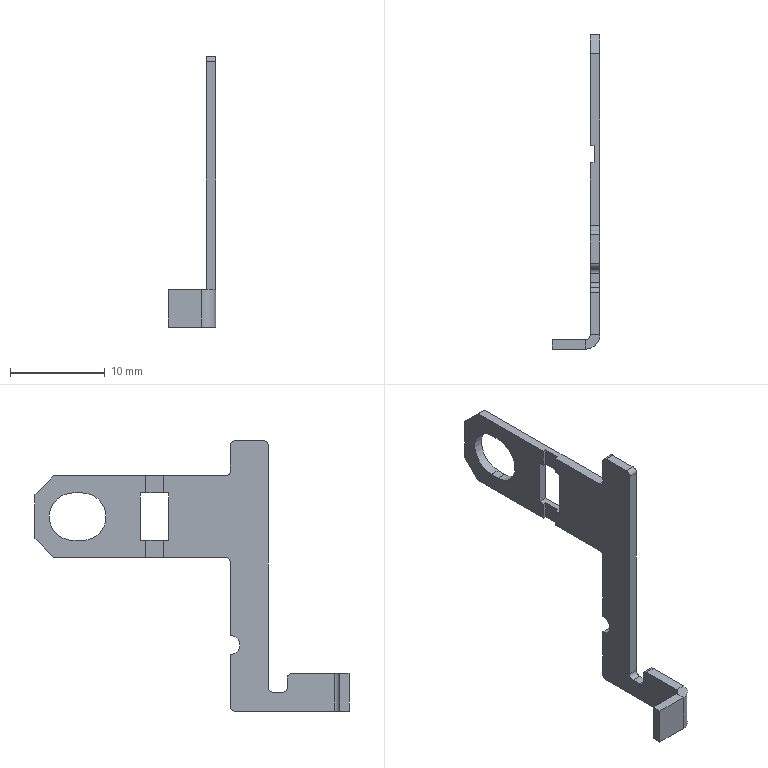Part | SolidWorks | features ICE 7, Chamfer 1, EdgeFlange 1, Fillet 1, FlatPattern 1, SMBaseFlange 1, SheetMetal 1 | 1 solid | 49 faces | box 5 x 33.1 x 28.5 mm | volume 287.645 mm3 | plane 36 | cylinder 13 | commonest cylinder face diameters 1 x9 5 x2 2 x1 3 x1
STEP:
#1=CARTESIAN_POINT('',(-4.,12.5,5.98));
#2=VERTEX_POINT('',#1);
#3=CARTESIAN_POINT('',(-5.,12.5,5.98));
#4=VERTEX_POINT('',#3);
#5=CARTESIAN_POINT('',(0.,12.5,5.98));
#6=DIRECTION('',(-1.,0.,0.));
#7=VECTOR('',#6,1000.);
#8=LINE('',#5,#7);
#9=EDGE_CURVE('',#2,#4,#8,.T.);
#10=ORIENTED_EDGE('',*,*,#9,.F.);
#11=CARTESIAN_POINT('',(-4.,12.5,0.5));
#12=VERTEX_POINT('',#11);
#13=CARTESIAN_POINT('',(-4.,12.5,4.));
#14=DIRECTION('',(0.,0.,-1.));
#15=VECTOR('',#14,1000.);
#16=LINE('',#13,#15);
#17=EDGE_CURVE('',#2,#12,#16,.T.);
#18=ORIENTED_EDGE('',*,*,#17,.T.);
#19=CARTESIAN_POINT('',(-5.,12.5,0.5));
#20=VERTEX_POINT('',#19);
#21=CARTESIAN_POINT('',(-5.,12.5,0.5));
#22=DIRECTION('',(-1.,0.,0.));
#23=VECTOR('',#22,1000.);
#24=LINE('',#21,#23);
#25=EDGE_CURVE('',#12,#20,#24,.T.);
#26=ORIENTED_EDGE('',*,*,#25,.T.);
#27=CARTESIAN_POINT('',(-5.,12.5,4.));
#28=DIRECTION('',(0.,0.,-1.));
#29=VECTOR('',#28,1000.);
#30=LINE('',#27,#29);
#31=EDGE_CURVE('',#4,#20,#30,.T.);
#32=ORIENTED_EDGE('',*,*,#31,.F.);
#33=EDGE_LOOP('',(#10,#18,#26,#32));
#34=FACE_OUTER_BOUND('',#33,.T.);
#35=CARTESIAN_POINT('',(-5.,12.5,4.));
#36=DIRECTION('',(0.,1.,0.));
#37=DIRECTION('',(0.,0.,1.));
#38=AXIS2_PLACEMENT_3D('',#35,#36,#37);
#39=PLANE('',#38);
#40=ADVANCED_FACE('',(#34),#39,.T.);
#41=CARTESIAN_POINT('',(-4.6,21.4,16.2));
#42=VERTEX_POINT('',#41);
#43=CARTESIAN_POINT('',(-4.6,21.4,18.));
#44=VERTEX_POINT('',#43);
#45=CARTESIAN_POINT('',(-4.6,21.4,0.));
#46=DIRECTION('',(0.,0.,1.));
#47=VECTOR('',#46,1000.);
#48=LINE('',#45,#47);
#49=EDGE_CURVE('',#42,#44,#48,.T.);
#50=ORIENTED_EDGE('',*,*,#49,.T.);
#51=CARTESIAN_POINT('',(-5.,21.4,18.));
#52=VERTEX_POINT('',#51);
#53=CARTESIAN_POINT('',(-5.,21.4,18.));
#54=DIRECTION('',(-1.,0.,0.));
#55=VECTOR('',#54,1000.);
#56=LINE('',#53,#55);
#57=EDGE_CURVE('',#44,#52,#56,.T.);
#58=ORIENTED_EDGE('',*,*,#57,.T.);
#59=CARTESIAN_POINT('',(-5.,21.4,16.2));
#60=VERTEX_POINT('',#59);
#61=CARTESIAN_POINT('',(-5.,21.4,0.));
#62=DIRECTION('',(0.,0.,1.));
#63=VECTOR('',#62,1000.);
#64=LINE('',#61,#63);
#65=EDGE_CURVE('',#60,#52,#64,.T.);
#66=ORIENTED_EDGE('',*,*,#65,.F.);
#67=CARTESIAN_POINT('',(18.323,21.4,16.2));
#68=DIRECTION('',(1.,0.,0.));
#69=VECTOR('',#68,1000.);
#70=LINE('',#67,#69);
#71=EDGE_CURVE('',#60,#42,#70,.T.);
#72=ORIENTED_EDGE('',*,*,#71,.T.);
#73=EDGE_LOOP('',(#50,#58,#66,#72));
#74=FACE_OUTER_BOUND('',#73,.T.);
#75=CARTESIAN_POINT('',(-5.,21.4,0.));
#76=DIRECTION('',(0.,1.,0.));
#77=DIRECTION('',(-1.,0.,0.));
#78=AXIS2_PLACEMENT_3D('',#75,#76,#77);
#79=PLANE('',#78);
#80=ADVANCED_FACE('',(#74),#79,.F.);
#81=CARTESIAN_POINT('',(-4.6,19.6,16.2));
#82=VERTEX_POINT('',#81);
#83=CARTESIAN_POINT('',(-4.6,19.6,18.));
#84=VERTEX_POINT('',#83);
#85=CARTESIAN_POINT('',(-4.6,19.6,0.));
#86=DIRECTION('',(0.,0.,1.));
#87=VECTOR('',#86,1000.);
#88=LINE('',#85,#87);
#89=EDGE_CURVE('',#82,#84,#88,.T.);
#90=ORIENTED_EDGE('',*,*,#89,.T.);
#91=CARTESIAN_POINT('',(-4.6,21.4,18.));
#92=DIRECTION('',(0.,1.,0.));
#93=VECTOR('',#92,1000.);
#94=LINE('',#91,#93);
#95=EDGE_CURVE('',#84,#44,#94,.T.);
#96=ORIENTED_EDGE('',*,*,#95,.T.);
#97=ORIENTED_EDGE('',*,*,#49,.F.);
#98=CARTESIAN_POINT('',(-4.6,12.5,16.2));
#99=DIRECTION('',(0.,-1.,0.));
#100=VECTOR('',#99,1000.);
#101=LINE('',#98,#100);
#102=EDGE_CURVE('',#42,#82,#101,.T.);
#103=ORIENTED_EDGE('',*,*,#102,.T.);
#104=EDGE_LOOP('',(#90,#96,#97,#103));
#105=FACE_OUTER_BOUND('',#104,.T.);
#106=CARTESIAN_POINT('',(-4.6,21.4,0.));
#107=DIRECTION('',(1.,0.,0.));
#108=DIRECTION('',(0.,0.,-1.));
#109=AXIS2_PLACEMENT_3D('',#106,#107,#108);
#110=PLANE('',#109);
#111=ADVANCED_FACE('',(#105),#110,.F.);
#112=CARTESIAN_POINT('',(-5.,19.6,16.2));
#113=VERTEX_POINT('',#112);
#114=CARTESIAN_POINT('',(-5.,19.6,18.));
#115=VERTEX_POINT('',#114);
#116=CARTESIAN_POINT('',(-5.,19.6,0.));
#117=DIRECTION('',(0.,0.,1.));
#118=VECTOR('',#117,1000.);
#119=LINE('',#116,#118);
#120=EDGE_CURVE('',#113,#115,#119,.T.);
#121=ORIENTED_EDGE('',*,*,#120,.T.);
#122=CARTESIAN_POINT('',(-5.,19.6,18.));
#123=DIRECTION('',(1.,0.,0.));
#124=VECTOR('',#123,1000.);
#125=LINE('',#122,#124);
#126=EDGE_CURVE('',#115,#84,#125,.T.);
#127=ORIENTED_EDGE('',*,*,#126,.T.);
#128=ORIENTED_EDGE('',*,*,#89,.F.);
#129=CARTESIAN_POINT('',(18.323,19.6,16.2));
#130=DIRECTION('',(-1.,0.,0.));
#131=VECTOR('',#130,1000.);
#132=LINE('',#129,#131);
#133=EDGE_CURVE('',#82,#113,#132,.T.);
#134=ORIENTED_EDGE('',*,*,#133,.T.);
#135=EDGE_LOOP('',(#121,#127,#128,#134));
#136=FACE_OUTER_BOUND('',#135,.T.);
#137=CARTESIAN_POINT('',(-5.,19.6,0.));
#138=DIRECTION('',(0.,-1.,0.));
#139=DIRECTION('',(0.,0.,-1.));
#140=AXIS2_PLACEMENT_3D('',#137,#138,#139);
#141=PLANE('',#140);
#142=ADVANCED_FACE('',(#136),#141,.F.);
#143=CARTESIAN_POINT('',(-5.,29.1,23.));
#144=VERTEX_POINT('',#143);
#145=CARTESIAN_POINT('',(-5.,29.1,18.));
#146=VERTEX_POINT('',#145);
#147=CARTESIAN_POINT('',(-5.,29.1,20.5));
#148=DIRECTION('',(-1.,0.,0.));
#149=DIRECTION('',(0.,0.,1.));
#150=AXIS2_PLACEMENT_3D('',#147,#148,#149);
#151=CIRCLE('',#150,2.5);
#152=EDGE_CURVE('',#144,#146,#151,.T.);
#153=ORIENTED_EDGE('',*,*,#152,.F.);
#154=CARTESIAN_POINT('',(-5.,28.1,23.));
#155=VERTEX_POINT('',#154);
#156=CARTESIAN_POINT('',(-5.,29.1,23.));
#157=DIRECTION('',(0.,1.,0.));
#158=VECTOR('',#157,1000.);
#159=LINE('',#156,#158);
#160=EDGE_CURVE('',#155,#144,#159,.T.);
#161=ORIENTED_EDGE('',*,*,#160,.F.);
#162=CARTESIAN_POINT('',(-5.,28.1,18.));
#163=VERTEX_POINT('',#162);
#164=CARTESIAN_POINT('',(-5.,28.1,20.5));
#165=DIRECTION('',(-1.,0.,0.));
#166=DIRECTION('',(0.,0.,1.));
#167=AXIS2_PLACEMENT_3D('',#164,#165,#166);
#168=CIRCLE('',#167,2.5);
#169=EDGE_CURVE('',#163,#155,#168,.T.);
#170=ORIENTED_EDGE('',*,*,#169,.F.);
#171=CARTESIAN_POINT('',(-5.,29.1,18.));
#172=DIRECTION('',(0.,-1.,0.));
#173=VECTOR('',#172,1000.);
#174=LINE('',#171,#173);
#175=EDGE_CURVE('',#146,#163,#174,.T.);
#176=ORIENTED_EDGE('',*,*,#175,.F.);
#177=EDGE_LOOP('',(#153,#161,#170,#176));
#178=FACE_BOUND('',#177,.T.);
#179=CARTESIAN_POINT('',(-5.,21.4,24.8));
#180=VERTEX_POINT('',#179);
#181=CARTESIAN_POINT('',(-5.,31.1,24.8));
#182=VERTEX_POINT('',#181);
#183=CARTESIAN_POINT('',(-5.,12.5,24.8));
#184=DIRECTION('',(0.,1.,0.));
#185=VECTOR('',#184,1000.);
#186=LINE('',#183,#185);
#187=EDGE_CURVE('',#180,#182,#186,.T.);
#188=ORIENTED_EDGE('',*,*,#187,.T.);
#189=CARTESIAN_POINT('',(-5.,33.1,22.8));
#190=VERTEX_POINT('',#189);
#191=CARTESIAN_POINT('',(-5.,25.95,29.95));
#192=DIRECTION('',(0.,0.7071,-0.7071));
#193=VECTOR('',#192,1000.);
#194=LINE('',#191,#193);
#195=EDGE_CURVE('',#182,#190,#194,.T.);
#196=ORIENTED_EDGE('',*,*,#195,.T.);
#197=CARTESIAN_POINT('',(-5.,33.1,18.2));
#198=VERTEX_POINT('',#197);
#199=CARTESIAN_POINT('',(-5.,33.1,16.2));
#200=DIRECTION('',(0.,0.,-1.));
#201=VECTOR('',#200,1000.);
#202=LINE('',#199,#201);
#203=EDGE_CURVE('',#190,#198,#202,.T.);
#204=ORIENTED_EDGE('',*,*,#203,.T.);
#205=CARTESIAN_POINT('',(-5.,31.1,16.2));
#206=VERTEX_POINT('',#205);
#207=CARTESIAN_POINT('',(-5.,9.45,-5.45));
#208=DIRECTION('',(0.,-0.7071,-0.7071));
#209=VECTOR('',#208,1000.);
#210=LINE('',#207,#209);
#211=EDGE_CURVE('',#198,#206,#210,.T.);
#212=ORIENTED_EDGE('',*,*,#211,.T.);
#213=CARTESIAN_POINT('',(-5.,12.5,16.2));
#214=DIRECTION('',(0.,-1.,0.));
#215=VECTOR('',#214,1000.);
#216=LINE('',#213,#215);
#217=EDGE_CURVE('',#206,#60,#216,.T.);
#218=ORIENTED_EDGE('',*,*,#217,.T.);
#219=ORIENTED_EDGE('',*,*,#65,.T.);
#220=CARTESIAN_POINT('',(-5.,22.,18.));
#221=VERTEX_POINT('',#220);
#222=CARTESIAN_POINT('',(-5.,22.,18.));
#223=DIRECTION('',(0.,-1.,0.));
#224=VECTOR('',#223,1000.);
#225=LINE('',#222,#224);
#226=EDGE_CURVE('',#221,#52,#225,.T.);
#227=ORIENTED_EDGE('',*,*,#226,.F.);
#228=CARTESIAN_POINT('',(-5.,22.,23.));
#229=VERTEX_POINT('',#228);
#230=CARTESIAN_POINT('',(-5.,22.,18.));
#231=DIRECTION('',(0.,0.,-1.));
#232=VECTOR('',#231,1000.);
#233=LINE('',#230,#232);
#234=EDGE_CURVE('',#229,#221,#233,.T.);
#235=ORIENTED_EDGE('',*,*,#234,.F.);
#236=CARTESIAN_POINT('',(-5.,21.4,23.));
#237=VERTEX_POINT('',#236);
#238=CARTESIAN_POINT('',(-5.,22.,23.));
#239=DIRECTION('',(0.,1.,0.));
#240=VECTOR('',#239,1000.);
#241=LINE('',#238,#240);
#242=EDGE_CURVE('',#237,#229,#241,.T.);
#243=ORIENTED_EDGE('',*,*,#242,.F.);
#244=CARTESIAN_POINT('',(-5.,21.4,0.));
#245=DIRECTION('',(0.,0.,1.));
#246=VECTOR('',#245,1000.);
#247=LINE('',#244,#246);
#248=EDGE_CURVE('',#237,#180,#247,.T.);
#249=ORIENTED_EDGE('',*,*,#248,.T.);
#250=EDGE_LOOP('',(#188,#196,#204,#212,#218,#219,#227,#235,#243,#249));
#251=FACE_OUTER_BOUND('',#250,.T.);
#252=CARTESIAN_POINT('',(-5.,0.,4.));
#253=DIRECTION('',(-1.,0.,0.));
#254=DIRECTION('',(0.,0.,1.));
#255=AXIS2_PLACEMENT_3D('',#252,#253,#254);
#256=PLANE('',#255);
#257=ADVANCED_FACE('',(#178,#251),#256,.T.);
#258=CARTESIAN_POINT('',(-5.,12.5,28.));
#259=VERTEX_POINT('',#258);
#260=CARTESIAN_POINT('',(-5.,12.5,25.3));
#261=VERTEX_POINT('',#260);
#262=CARTESIAN_POINT('',(-5.,12.5,4.));
#263=DIRECTION('',(0.,0.,-1.));
#264=VECTOR('',#263,1000.);
#265=LINE('',#262,#264);
#266=EDGE_CURVE('',#259,#261,#265,.T.);
#267=ORIENTED_EDGE('',*,*,#266,.F.);
#268=CARTESIAN_POINT('',(-4.,12.5,28.));
#269=VERTEX_POINT('',#268);
#270=CARTESIAN_POINT('',(-5.,12.5,28.));
#271=DIRECTION('',(1.,0.,0.));
#272=VECTOR('',#271,1000.);
#273=LINE('',#270,#272);
#274=EDGE_CURVE('',#259,#269,#273,.T.);
#275=ORIENTED_EDGE('',*,*,#274,.T.);
#276=CARTESIAN_POINT('',(-4.,12.5,25.3));
#277=VERTEX_POINT('',#276);
#278=CARTESIAN_POINT('',(-4.,12.5,4.));
#279=DIRECTION('',(0.,0.,-1.));
#280=VECTOR('',#279,1000.);
#281=LINE('',#278,#280);
#282=EDGE_CURVE('',#269,#277,#281,.T.);
#283=ORIENTED_EDGE('',*,*,#282,.T.);
#284=CARTESIAN_POINT('',(-5.,12.5,25.3));
#285=DIRECTION('',(-1.,0.,0.));
#286=VECTOR('',#285,1000.);
#287=LINE('',#284,#286);
#288=EDGE_CURVE('',#277,#261,#287,.T.);
#289=ORIENTED_EDGE('',*,*,#288,.T.);
#290=EDGE_LOOP('',(#267,#275,#283,#289));
#291=FACE_OUTER_BOUND('',#290,.T.);
#292=CARTESIAN_POINT('',(-5.,12.5,4.));
#293=DIRECTION('',(0.,1.,0.));
#294=DIRECTION('',(0.,0.,1.));
#295=AXIS2_PLACEMENT_3D('',#292,#293,#294);
#296=PLANE('',#295);
#297=ADVANCED_FACE('',(#291),#296,.T.);
#298=CARTESIAN_POINT('',(-4.,1.5,4.));
#299=VERTEX_POINT('',#298);
#300=CARTESIAN_POINT('',(-4.,6.,4.));
#301=VERTEX_POINT('',#300);
#302=CARTESIAN_POINT('',(-4.,0.,4.));
#303=DIRECTION('',(0.,1.,0.));
#304=VECTOR('',#303,1000.);
#305=LINE('',#302,#304);
#306=EDGE_CURVE('',#299,#301,#305,.T.);
#307=ORIENTED_EDGE('',*,*,#306,.T.);
#308=CARTESIAN_POINT('',(-5.,6.,4.));
#309=VERTEX_POINT('',#308);
#310=CARTESIAN_POINT('',(-5.,6.,4.));
#311=DIRECTION('',(-1.,0.,0.));
#312=VECTOR('',#311,1000.);
#313=LINE('',#310,#312);
#314=EDGE_CURVE('',#301,#309,#313,.T.);
#315=ORIENTED_EDGE('',*,*,#314,.T.);
#316=CARTESIAN_POINT('',(-5.,1.5,4.));
#317=VERTEX_POINT('',#316);
#318=CARTESIAN_POINT('',(-5.,0.,4.));
#319=DIRECTION('',(0.,1.,0.));
#320=VECTOR('',#319,1000.);
#321=LINE('',#318,#320);
#322=EDGE_CURVE('',#317,#309,#321,.T.);
#323=ORIENTED_EDGE('',*,*,#322,.F.);
#324=CARTESIAN_POINT('',(-5.,1.5,4.));
#325=DIRECTION('',(1.,0.,0.));
#326=VECTOR('',#325,1000.);
#327=LINE('',#324,#326);
#328=EDGE_CURVE('',#317,#299,#327,.T.);
#329=ORIENTED_EDGE('',*,*,#328,.T.);
#330=EDGE_LOOP('',(#307,#315,#323,#329));
#331=FACE_OUTER_BOUND('',#330,.T.);
#332=CARTESIAN_POINT('',(-3.5,1.,4.));
#333=DIRECTION('',(0.,0.,1.));
#334=DIRECTION('',(1.,0.,0.));
#335=AXIS2_PLACEMENT_3D('',#332,#333,#334);
#336=PLANE('',#335);
#337=ADVANCED_FACE('',(#331),#336,.T.);
#338=CARTESIAN_POINT('',(-4.,28.1,23.));
#339=VERTEX_POINT('',#338);
#340=CARTESIAN_POINT('',(-4.,29.1,23.));
#341=VERTEX_POINT('',#340);
#342=CARTESIAN_POINT('',(-4.,0.,23.));
#343=DIRECTION('',(0.,1.,0.));
#344=VECTOR('',#343,1000.);
#345=LINE('',#342,#344);
#346=EDGE_CURVE('',#339,#341,#345,.T.);
#347=ORIENTED_EDGE('',*,*,#346,.T.);
#348=CARTESIAN_POINT('',(-4.,29.1,18.));
#349=VERTEX_POINT('',#348);
#350=CARTESIAN_POINT('',(-4.,29.1,20.5));
#351=DIRECTION('',(-1.,0.,0.));
#352=DIRECTION('',(0.,0.,1.));
#353=AXIS2_PLACEMENT_3D('',#350,#351,#352);
#354=CIRCLE('',#353,2.5);
#355=EDGE_CURVE('',#341,#349,#354,.T.);
#356=ORIENTED_EDGE('',*,*,#355,.T.);
#357=CARTESIAN_POINT('',(-4.,28.1,18.));
#358=VERTEX_POINT('',#357);
#359=CARTESIAN_POINT('',(-4.,0.,18.));
#360=DIRECTION('',(0.,-1.,0.));
#361=VECTOR('',#360,1000.);
#362=LINE('',#359,#361);
#363=EDGE_CURVE('',#349,#358,#362,.T.);
#364=ORIENTED_EDGE('',*,*,#363,.T.);
#365=CARTESIAN_POINT('',(-4.,28.1,20.5));
#366=DIRECTION('',(-1.,0.,0.));
#367=DIRECTION('',(0.,0.,1.));
#368=AXIS2_PLACEMENT_3D('',#365,#366,#367);
#369=CIRCLE('',#368,2.5);
#370=EDGE_CURVE('',#358,#339,#369,.T.);
#371=ORIENTED_EDGE('',*,*,#370,.T.);
#372=EDGE_LOOP('',(#347,#356,#364,#371));
#373=FACE_BOUND('',#372,.T.);
#374=CARTESIAN_POINT('',(-4.,22.,23.));
#375=VERTEX_POINT('',#374);
#376=CARTESIAN_POINT('',(-4.,22.,18.));
#377=VERTEX_POINT('',#376);
#378=CARTESIAN_POINT('',(-4.,22.,4.));
#379=DIRECTION('',(0.,0.,-1.));
#380=VECTOR('',#379,1000.);
#381=LINE('',#378,#380);
#382=EDGE_CURVE('',#375,#377,#381,.T.);
#383=ORIENTED_EDGE('',*,*,#382,.T.);
#384=CARTESIAN_POINT('',(-4.,19.,18.));
#385=VERTEX_POINT('',#384);
#386=CARTESIAN_POINT('',(-4.,0.,18.));
#387=DIRECTION('',(0.,-1.,0.));
#388=VECTOR('',#387,1000.);
#389=LINE('',#386,#388);
#390=EDGE_CURVE('',#377,#385,#389,.T.);
#391=ORIENTED_EDGE('',*,*,#390,.T.);
#392=CARTESIAN_POINT('',(-4.,19.,23.));
#393=VERTEX_POINT('',#392);
#394=CARTESIAN_POINT('',(-4.,19.,4.));
#395=DIRECTION('',(0.,0.,1.));
#396=VECTOR('',#395,1000.);
#397=LINE('',#394,#396);
#398=EDGE_CURVE('',#385,#393,#397,.T.);
#399=ORIENTED_EDGE('',*,*,#398,.T.);
#400=CARTESIAN_POINT('',(-4.,0.,23.));
#401=DIRECTION('',(0.,1.,0.));
#402=VECTOR('',#401,1000.);
#403=LINE('',#400,#402);
#404=EDGE_CURVE('',#393,#375,#403,.T.);
#405=ORIENTED_EDGE('',*,*,#404,.T.);
#406=EDGE_LOOP('',(#383,#391,#399,#405));
#407=FACE_BOUND('',#406,.T.);
#408=ORIENTED_EDGE('',*,*,#17,.F.);
#409=CARTESIAN_POINT('',(-4.,12.5,7.98));
#410=VERTEX_POINT('',#409);
#411=CARTESIAN_POINT('',(-4.,12.5,6.98));
#412=DIRECTION('',(-1.,0.,0.));
#413=DIRECTION('',(0.,0.,1.));
#414=AXIS2_PLACEMENT_3D('',#411,#412,#413);
#415=CIRCLE('',#414,1.);
#416=EDGE_CURVE('',#2,#410,#415,.T.);
#417=ORIENTED_EDGE('',*,*,#416,.T.);
#418=CARTESIAN_POINT('',(-4.,12.5,15.7));
#419=VERTEX_POINT('',#418);
#420=CARTESIAN_POINT('',(-4.,12.5,4.));
#421=DIRECTION('',(0.,0.,-1.));
#422=VECTOR('',#421,1000.);
#423=LINE('',#420,#422);
#424=EDGE_CURVE('',#419,#410,#423,.T.);
#425=ORIENTED_EDGE('',*,*,#424,.F.);
#426=CARTESIAN_POINT('',(-4.,13.,16.2));
#427=VERTEX_POINT('',#426);
#428=CARTESIAN_POINT('',(-4.,13.,15.7));
#429=DIRECTION('',(-1.,0.,0.));
#430=DIRECTION('',(0.,0.,1.));
#431=AXIS2_PLACEMENT_3D('',#428,#429,#430);
#432=CIRCLE('',#431,0.5);
#433=EDGE_CURVE('',#419,#427,#432,.T.);
#434=ORIENTED_EDGE('',*,*,#433,.T.);
#435=CARTESIAN_POINT('',(-4.,31.1,16.2));
#436=VERTEX_POINT('',#435);
#437=CARTESIAN_POINT('',(-4.,12.5,16.2));
#438=DIRECTION('',(0.,1.,0.));
#439=VECTOR('',#438,1000.);
#440=LINE('',#437,#439);
#441=EDGE_CURVE('',#427,#436,#440,.T.);
#442=ORIENTED_EDGE('',*,*,#441,.T.);
#443=CARTESIAN_POINT('',(-4.,33.1,18.2));
#444=VERTEX_POINT('',#443);
#445=CARTESIAN_POINT('',(-4.,33.1,18.2));
#446=DIRECTION('',(0.,0.7071,0.7071));
#447=VECTOR('',#446,1000.);
#448=LINE('',#445,#447);
#449=EDGE_CURVE('',#436,#444,#448,.T.);
#450=ORIENTED_EDGE('',*,*,#449,.T.);
#451=CARTESIAN_POINT('',(-4.,33.1,22.8));
#452=VERTEX_POINT('',#451);
#453=CARTESIAN_POINT('',(-4.,33.1,16.2));
#454=DIRECTION('',(0.,0.,1.));
#455=VECTOR('',#454,1000.);
#456=LINE('',#453,#455);
#457=EDGE_CURVE('',#444,#452,#456,.T.);
#458=ORIENTED_EDGE('',*,*,#457,.T.);
#459=CARTESIAN_POINT('',(-4.,31.1,24.8));
#460=VERTEX_POINT('',#459);
#461=CARTESIAN_POINT('',(-4.,31.1,24.8));
#462=DIRECTION('',(0.,-0.7071,0.7071));
#463=VECTOR('',#462,1000.);
#464=LINE('',#461,#463);
#465=EDGE_CURVE('',#452,#460,#464,.T.);
#466=ORIENTED_EDGE('',*,*,#465,.T.);
#467=CARTESIAN_POINT('',(-4.,13.,24.8));
#468=VERTEX_POINT('',#467);
#469=CARTESIAN_POINT('',(-4.,12.5,24.8));
#470=DIRECTION('',(0.,-1.,0.));
#471=VECTOR('',#470,1000.);
#472=LINE('',#469,#471);
#473=EDGE_CURVE('',#460,#468,#472,.T.);
#474=ORIENTED_EDGE('',*,*,#473,.T.);
#475=CARTESIAN_POINT('',(-4.,13.,25.3));
#476=DIRECTION('',(-1.,0.,0.));
#477=DIRECTION('',(0.,0.,1.));
#478=AXIS2_PLACEMENT_3D('',#475,#476,#477);
#479=CIRCLE('',#478,0.5);
#480=EDGE_CURVE('',#468,#277,#479,.T.);
#481=ORIENTED_EDGE('',*,*,#480,.T.);
#482=ORIENTED_EDGE('',*,*,#282,.F.);
#483=CARTESIAN_POINT('',(-4.,12.,28.5));
#484=VERTEX_POINT('',#483);
#485=CARTESIAN_POINT('',(-4.,12.,28.));
#486=DIRECTION('',(1.,0.,0.));
#487=DIRECTION('',(0.,0.,1.));
#488=AXIS2_PLACEMENT_3D('',#485,#486,#487);
#489=CIRCLE('',#488,0.5);
#490=EDGE_CURVE('',#269,#484,#489,.T.);
#491=ORIENTED_EDGE('',*,*,#490,.T.);
#492=CARTESIAN_POINT('',(-4.,9.,28.5));
#493=VERTEX_POINT('',#492);
#494=CARTESIAN_POINT('',(-4.,8.5,28.5));
#495=DIRECTION('',(0.,1.,0.));
#496=VECTOR('',#495,1000.);
#497=LINE('',#494,#496);
#498=EDGE_CURVE('',#493,#484,#497,.T.);
#499=ORIENTED_EDGE('',*,*,#498,.F.);
#500=CARTESIAN_POINT('',(-4.,8.5,28.));
#501=VERTEX_POINT('',#500);
#502=CARTESIAN_POINT('',(-4.,9.,28.));
#503=DIRECTION('',(1.,0.,0.));
#504=DIRECTION('',(0.,0.,1.));
#505=AXIS2_PLACEMENT_3D('',#502,#503,#504);
#506=CIRCLE('',#505,0.5);
#507=EDGE_CURVE('',#493,#501,#506,.T.);
#508=ORIENTED_EDGE('',*,*,#507,.T.);
#509=CARTESIAN_POINT('',(-4.,8.5,2.5));
#510=VERTEX_POINT('',#509);
#511=CARTESIAN_POINT('',(-4.,8.5,4.));
#512=DIRECTION('',(0.,0.,-1.));
#513=VECTOR('',#512,1000.);
#514=LINE('',#511,#513);
#515=EDGE_CURVE('',#501,#510,#514,.T.);
#516=ORIENTED_EDGE('',*,*,#515,.T.);
#517=CARTESIAN_POINT('',(-4.,8.,2.));
#518=VERTEX_POINT('',#517);
#519=CARTESIAN_POINT('',(-4.,8.,2.5));
#520=DIRECTION('',(-1.,0.,0.));
#521=DIRECTION('',(0.,0.,1.));
#522=AXIS2_PLACEMENT_3D('',#519,#520,#521);
#523=CIRCLE('',#522,0.5);
#524=EDGE_CURVE('',#510,#518,#523,.T.);
#525=ORIENTED_EDGE('',*,*,#524,.T.);
#526=CARTESIAN_POINT('',(-4.,7.,2.));
#527=VERTEX_POINT('',#526);
#528=CARTESIAN_POINT('',(-4.,0.,2.));
#529=DIRECTION('',(0.,-1.,0.));
#530=VECTOR('',#529,1000.);
#531=LINE('',#528,#530);
#532=EDGE_CURVE('',#518,#527,#531,.T.);
#533=ORIENTED_EDGE('',*,*,#532,.T.);
#534=CARTESIAN_POINT('',(-4.,6.5,2.5));
#535=VERTEX_POINT('',#534);
#536=CARTESIAN_POINT('',(-4.,7.,2.5));
#537=DIRECTION('',(-1.,0.,0.));
#538=DIRECTION('',(0.,0.,1.));
#539=AXIS2_PLACEMENT_3D('',#536,#537,#538);
#540=CIRCLE('',#539,0.5);
#541=EDGE_CURVE('',#527,#535,#540,.T.);
#542=ORIENTED_EDGE('',*,*,#541,.T.);
#543=CARTESIAN_POINT('',(-4.,6.5,3.5));
#544=VERTEX_POINT('',#543);
#545=CARTESIAN_POINT('',(-4.,6.5,4.));
#546=DIRECTION('',(0.,0.,1.));
#547=VECTOR('',#546,1000.);
#548=LINE('',#545,#547);
#549=EDGE_CURVE('',#535,#544,#548,.T.);
#550=ORIENTED_EDGE('',*,*,#549,.T.);
#551=CARTESIAN_POINT('',(-4.,6.,3.5));
#552=DIRECTION('',(1.,0.,0.));
#553=DIRECTION('',(0.,0.,1.));
#554=AXIS2_PLACEMENT_3D('',#551,#552,#553);
#555=CIRCLE('',#554,0.5);
#556=EDGE_CURVE('',#544,#301,#555,.T.);
#557=ORIENTED_EDGE('',*,*,#556,.T.);
#558=ORIENTED_EDGE('',*,*,#306,.F.);
#559=CARTESIAN_POINT('',(-4.,1.5,0.));
#560=VERTEX_POINT('',#559);
#561=CARTESIAN_POINT('',(-4.,1.5,4.));
#562=DIRECTION('',(0.,0.,-1.));
#563=VECTOR('',#562,1000.);
#564=LINE('',#561,#563);
#565=EDGE_CURVE('',#299,#560,#564,.T.);
#566=ORIENTED_EDGE('',*,*,#565,.T.);
#567=CARTESIAN_POINT('',(-4.,12.,0.));
#568=VERTEX_POINT('',#567);
#569=CARTESIAN_POINT('',(-4.,0.,0.));
#570=DIRECTION('',(0.,1.,0.));
#571=VECTOR('',#570,1000.);
#572=LINE('',#569,#571);
#573=EDGE_CURVE('',#560,#568,#572,.T.);
#574=ORIENTED_EDGE('',*,*,#573,.T.);
#575=CARTESIAN_POINT('',(-4.,12.,0.5));
#576=DIRECTION('',(1.,0.,0.));
#577=DIRECTION('',(0.,0.,1.));
#578=AXIS2_PLACEMENT_3D('',#575,#576,#577);
#579=CIRCLE('',#578,0.5);
#580=EDGE_CURVE('',#568,#12,#579,.T.);
#581=ORIENTED_EDGE('',*,*,#580,.T.);
#582=EDGE_LOOP('',(#408,#417,#425,#434,#442,#450,#458,#466,#474,#481,#482,#491,#499,#508,#516,#525,#533,#542,#550,#557,#558,#566,#574,#581));
#583=FACE_OUTER_BOUND('',#582,.T.);
#584=CARTESIAN_POINT('',(-4.,0.,4.));
#585=DIRECTION('',(-1.,0.,0.));
#586=DIRECTION('',(0.,0.,1.));
#587=AXIS2_PLACEMENT_3D('',#584,#585,#586);
#588=PLANE('',#587);
#589=ADVANCED_FACE('',(#373,#407,#583),#588,.F.);
#590=CARTESIAN_POINT('',(-5.,12.5,7.98));
#591=VERTEX_POINT('',#590);
#592=CARTESIAN_POINT('',(0.,12.5,7.98));
#593=DIRECTION('',(1.,0.,0.));
#594=VECTOR('',#593,1000.);
#595=LINE('',#592,#594);
#596=EDGE_CURVE('',#591,#410,#595,.T.);
#597=ORIENTED_EDGE('',*,*,#596,.F.);
#598=CARTESIAN_POINT('',(-5.,12.5,15.7));
#599=VERTEX_POINT('',#598);
#600=CARTESIAN_POINT('',(-5.,12.5,4.));
#601=DIRECTION('',(0.,0.,-1.));
#602=VECTOR('',#601,1000.);
#603=LINE('',#600,#602);
#604=EDGE_CURVE('',#599,#591,#603,.T.);
#605=ORIENTED_EDGE('',*,*,#604,.F.);
#606=CARTESIAN_POINT('',(-4.,12.5,15.7));
#607=DIRECTION('',(1.,0.,0.));
#608=VECTOR('',#607,1000.);
#609=LINE('',#606,#608);
#610=EDGE_CURVE('',#599,#419,#609,.T.);
#611=ORIENTED_EDGE('',*,*,#610,.T.);
#612=ORIENTED_EDGE('',*,*,#424,.T.);
#613=EDGE_LOOP('',(#597,#605,#611,#612));
#614=FACE_OUTER_BOUND('',#613,.T.);
#615=CARTESIAN_POINT('',(-5.,12.5,4.));
#616=DIRECTION('',(0.,1.,0.));
#617=DIRECTION('',(0.,0.,1.));
#618=AXIS2_PLACEMENT_3D('',#615,#616,#617);
#619=PLANE('',#618);
#620=ADVANCED_FACE('',(#614),#619,.T.);
#621=CARTESIAN_POINT('',(-5.,12.5,6.98));
#622=DIRECTION('',(-1.,0.,0.));
#623=DIRECTION('',(0.,0.,1.));
#624=AXIS2_PLACEMENT_3D('',#621,#622,#623);
#625=CIRCLE('',#624,1.);
#626=EDGE_CURVE('',#4,#591,#625,.T.);
#627=ORIENTED_EDGE('',*,*,#626,.F.);
#628=ORIENTED_EDGE('',*,*,#31,.T.);
#629=CARTESIAN_POINT('',(-5.,12.,0.));
#630=VERTEX_POINT('',#629);
#631=CARTESIAN_POINT('',(-5.,12.,0.5));
#632=DIRECTION('',(-1.,0.,0.));
#633=DIRECTION('',(0.,0.,1.));
#634=AXIS2_PLACEMENT_3D('',#631,#632,#633);
#635=CIRCLE('',#634,0.5);
#636=EDGE_CURVE('',#20,#630,#635,.T.);
#637=ORIENTED_EDGE('',*,*,#636,.T.);
#638=CARTESIAN_POINT('',(-5.,1.5,0.));
#639=VERTEX_POINT('',#638);
#640=CARTESIAN_POINT('',(-5.,0.,0.));
#641=DIRECTION('',(0.,1.,0.));
#642=VECTOR('',#641,1000.);
#643=LINE('',#640,#642);
#644=EDGE_CURVE('',#639,#630,#643,.T.);
#645=ORIENTED_EDGE('',*,*,#644,.F.);
#646=CARTESIAN_POINT('',(-5.,1.5,4.));
#647=DIRECTION('',(0.,0.,-1.));
#648=VECTOR('',#647,1000.);
#649=LINE('',#646,#648);
#650=EDGE_CURVE('',#317,#639,#649,.T.);
#651=ORIENTED_EDGE('',*,*,#650,.F.);
#652=ORIENTED_EDGE('',*,*,#322,.T.);
#653=CARTESIAN_POINT('',(-5.,6.5,3.5));
#654=VERTEX_POINT('',#653);
#655=CARTESIAN_POINT('',(-5.,6.,3.5));
#656=DIRECTION('',(-1.,0.,0.));
#657=DIRECTION('',(0.,0.,1.));
#658=AXIS2_PLACEMENT_3D('',#655,#656,#657);
#659=CIRCLE('',#658,0.5);
#660=EDGE_CURVE('',#309,#654,#659,.T.);
#661=ORIENTED_EDGE('',*,*,#660,.T.);
#662=CARTESIAN_POINT('',(-5.,6.5,2.5));
#663=VERTEX_POINT('',#662);
#664=CARTESIAN_POINT('',(-5.,6.5,2.));
#665=DIRECTION('',(0.,0.,1.));
#666=VECTOR('',#665,1000.);
#667=LINE('',#664,#666);
#668=EDGE_CURVE('',#663,#654,#667,.T.);
#669=ORIENTED_EDGE('',*,*,#668,.F.);
#670=CARTESIAN_POINT('',(-5.,7.,2.));
#671=VERTEX_POINT('',#670);
#672=CARTESIAN_POINT('',(-5.,7.,2.5));
#673=DIRECTION('',(1.,0.,0.));
#674=DIRECTION('',(0.,0.,1.));
#675=AXIS2_PLACEMENT_3D('',#672,#673,#674);
#676=CIRCLE('',#675,0.5);
#677=EDGE_CURVE('',#663,#671,#676,.T.);
#678=ORIENTED_EDGE('',*,*,#677,.T.);
#679=CARTESIAN_POINT('',(-5.,8.,2.));
#680=VERTEX_POINT('',#679);
#681=CARTESIAN_POINT('',(-5.,8.5,2.));
#682=DIRECTION('',(0.,-1.,0.));
#683=VECTOR('',#682,1000.);
#684=LINE('',#681,#683);
#685=EDGE_CURVE('',#680,#671,#684,.T.);
#686=ORIENTED_EDGE('',*,*,#685,.F.);
#687=CARTESIAN_POINT('',(-5.,8.5,2.5));
#688=VERTEX_POINT('',#687);
#689=CARTESIAN_POINT('',(-5.,8.,2.5));
#690=DIRECTION('',(1.,0.,0.));
#691=DIRECTION('',(0.,0.,1.));
#692=AXIS2_PLACEMENT_3D('',#689,#690,#691);
#693=CIRCLE('',#692,0.5);
#694=EDGE_CURVE('',#680,#688,#693,.T.);
#695=ORIENTED_EDGE('',*,*,#694,.T.);
#696=CARTESIAN_POINT('',(-5.,8.5,28.));
#697=VERTEX_POINT('',#696);
#698=CARTESIAN_POINT('',(-5.,8.5,4.));
#699=DIRECTION('',(0.,0.,1.));
#700=VECTOR('',#699,1000.);
#701=LINE('',#698,#700);
#702=EDGE_CURVE('',#688,#697,#701,.T.);
#703=ORIENTED_EDGE('',*,*,#702,.T.);
#704=CARTESIAN_POINT('',(-5.,9.,28.5));
#705=VERTEX_POINT('',#704);
#706=CARTESIAN_POINT('',(-5.,9.,28.));
#707=DIRECTION('',(-1.,0.,0.));
#708=DIRECTION('',(0.,0.,1.));
#709=AXIS2_PLACEMENT_3D('',#706,#707,#708);
#710=CIRCLE('',#709,0.5);
#711=EDGE_CURVE('',#697,#705,#710,.T.);
#712=ORIENTED_EDGE('',*,*,#711,.T.);
#713=CARTESIAN_POINT('',(-5.,12.,28.5));
#714=VERTEX_POINT('',#713);
#715=CARTESIAN_POINT('',(-5.,8.5,28.5));
#716=DIRECTION('',(0.,1.,0.));
#717=VECTOR('',#716,1000.);
#718=LINE('',#715,#717);
#719=EDGE_CURVE('',#705,#714,#718,.T.);
#720=ORIENTED_EDGE('',*,*,#719,.T.);
#721=CARTESIAN_POINT('',(-5.,12.,28.));
#722=DIRECTION('',(-1.,0.,0.));
#723=DIRECTION('',(0.,0.,1.));
#724=AXIS2_PLACEMENT_3D('',#721,#722,#723);
#725=CIRCLE('',#724,0.5);
#726=EDGE_CURVE('',#714,#259,#725,.T.);
#727=ORIENTED_EDGE('',*,*,#726,.T.);
#728=ORIENTED_EDGE('',*,*,#266,.T.);
#729=CARTESIAN_POINT('',(-5.,13.,24.8));
#730=VERTEX_POINT('',#729);
#731=CARTESIAN_POINT('',(-5.,13.,25.3));
#732=DIRECTION('',(1.,0.,0.));
#733=DIRECTION('',(0.,0.,1.));
#734=AXIS2_PLACEMENT_3D('',#731,#732,#733);
#735=CIRCLE('',#734,0.5);
#736=EDGE_CURVE('',#261,#730,#735,.T.);
#737=ORIENTED_EDGE('',*,*,#736,.T.);
#738=CARTESIAN_POINT('',(-5.,19.6,24.8));
#739=VERTEX_POINT('',#738);
#740=CARTESIAN_POINT('',(-5.,12.5,24.8));
#741=DIRECTION('',(0.,1.,0.));
#742=VECTOR('',#741,1000.);
#743=LINE('',#740,#742);
#744=EDGE_CURVE('',#730,#739,#743,.T.);
#745=ORIENTED_EDGE('',*,*,#744,.T.);
#746=CARTESIAN_POINT('',(-5.,19.6,23.));
#747=VERTEX_POINT('',#746);
#748=CARTESIAN_POINT('',(-5.,19.6,0.));
#749=DIRECTION('',(0.,0.,1.));
#750=VECTOR('',#749,1000.);
#751=LINE('',#748,#750);
#752=EDGE_CURVE('',#747,#739,#751,.T.);
#753=ORIENTED_EDGE('',*,*,#752,.F.);
#754=CARTESIAN_POINT('',(-5.,19.,23.));
#755=VERTEX_POINT('',#754);
#756=CARTESIAN_POINT('',(-5.,22.,23.));
#757=DIRECTION('',(0.,1.,0.));
#758=VECTOR('',#757,1000.);
#759=LINE('',#756,#758);
#760=EDGE_CURVE('',#755,#747,#759,.T.);
#761=ORIENTED_EDGE('',*,*,#760,.F.);
#762=CARTESIAN_POINT('',(-5.,19.,18.));
#763=VERTEX_POINT('',#762);
#764=CARTESIAN_POINT('',(-5.,19.,18.));
#765=DIRECTION('',(0.,0.,1.));
#766=VECTOR('',#765,1000.);
#767=LINE('',#764,#766);
#768=EDGE_CURVE('',#763,#755,#767,.T.);
#769=ORIENTED_EDGE('',*,*,#768,.F.);
#770=CARTESIAN_POINT('',(-5.,22.,18.));
#771=DIRECTION('',(0.,-1.,0.));
#772=VECTOR('',#771,1000.);
#773=LINE('',#770,#772);
#774=EDGE_CURVE('',#115,#763,#773,.T.);
#775=ORIENTED_EDGE('',*,*,#774,.F.);
#776=ORIENTED_EDGE('',*,*,#120,.F.);
#777=CARTESIAN_POINT('',(-5.,13.,16.2));
#778=VERTEX_POINT('',#777);
#779=CARTESIAN_POINT('',(-5.,12.5,16.2));
#780=DIRECTION('',(0.,-1.,0.));
#781=VECTOR('',#780,1000.);
#782=LINE('',#779,#781);
#783=EDGE_CURVE('',#113,#778,#782,.T.);
#784=ORIENTED_EDGE('',*,*,#783,.T.);
#785=CARTESIAN_POINT('',(-5.,13.,15.7));
#786=DIRECTION('',(1.,0.,0.));
#787=DIRECTION('',(0.,0.,1.));
#788=AXIS2_PLACEMENT_3D('',#785,#786,#787);
#789=CIRCLE('',#788,0.5);
#790=EDGE_CURVE('',#778,#599,#789,.T.);
#791=ORIENTED_EDGE('',*,*,#790,.T.);
#792=ORIENTED_EDGE('',*,*,#604,.T.);
#793=EDGE_LOOP('',(#627,#628,#637,#645,#651,#652,#661,#669,#678,#686,#695,#703,#712,#720,#727,#728,#737,#745,#753,#761,#769,#775,#776,#784,#791,#792));
#794=FACE_OUTER_BOUND('',#793,.T.);
#795=CARTESIAN_POINT('',(-5.,0.,4.));
#796=DIRECTION('',(-1.,0.,0.));
#797=DIRECTION('',(0.,0.,1.));
#798=AXIS2_PLACEMENT_3D('',#795,#796,#797);
#799=PLANE('',#798);
#800=ADVANCED_FACE('',(#794),#799,.T.);
#801=ORIENTED_EDGE('',*,*,#644,.T.);
#802=CARTESIAN_POINT('',(-4.,12.,0.));
#803=DIRECTION('',(1.,0.,0.));
#804=VECTOR('',#803,1000.);
#805=LINE('',#802,#804);
#806=EDGE_CURVE('',#630,#568,#805,.T.);
#807=ORIENTED_EDGE('',*,*,#806,.T.);
#808=ORIENTED_EDGE('',*,*,#573,.F.);
#809=CARTESIAN_POINT('',(-4.,1.5,0.));
#810=DIRECTION('',(-1.,0.,0.));
#811=VECTOR('',#810,1000.);
#812=LINE('',#809,#811);
#813=EDGE_CURVE('',#560,#639,#812,.T.);
#814=ORIENTED_EDGE('',*,*,#813,.T.);
#815=EDGE_LOOP('',(#801,#807,#808,#814));
#816=FACE_OUTER_BOUND('',#815,.T.);
#817=CARTESIAN_POINT('',(-3.5,1.5,0.));
#818=DIRECTION('',(0.,0.,1.));
#819=DIRECTION('',(1.,0.,0.));
#820=AXIS2_PLACEMENT_3D('',#817,#818,#819);
#821=PLANE('',#820);
#822=ADVANCED_FACE('',(#816),#821,.F.);
#823=ORIENTED_EDGE('',*,*,#719,.F.);
#824=CARTESIAN_POINT('',(-4.,9.,28.5));
#825=DIRECTION('',(1.,0.,0.));
#826=VECTOR('',#825,1000.);
#827=LINE('',#824,#826);
#828=EDGE_CURVE('',#705,#493,#827,.T.);
#829=ORIENTED_EDGE('',*,*,#828,.T.);
#830=ORIENTED_EDGE('',*,*,#498,.T.);
#831=CARTESIAN_POINT('',(-5.,12.,28.5));
#832=DIRECTION('',(-1.,0.,0.));
#833=VECTOR('',#832,1000.);
#834=LINE('',#831,#833);
#835=EDGE_CURVE('',#484,#714,#834,.T.);
#836=ORIENTED_EDGE('',*,*,#835,.T.);
#837=EDGE_LOOP('',(#823,#829,#830,#836));
#838=FACE_OUTER_BOUND('',#837,.T.);
#839=CARTESIAN_POINT('',(-5.,8.5,28.5));
#840=DIRECTION('',(0.,0.,1.));
#841=DIRECTION('',(1.,0.,0.));
#842=AXIS2_PLACEMENT_3D('',#839,#840,#841);
#843=PLANE('',#842);
#844=ADVANCED_FACE('',(#838),#843,.T.);
#845=ORIENTED_EDGE('',*,*,#515,.F.);
#846=CARTESIAN_POINT('',(-5.,8.5,28.));
#847=DIRECTION('',(-1.,0.,0.));
#848=VECTOR('',#847,1000.);
#849=LINE('',#846,#848);
#850=EDGE_CURVE('',#501,#697,#849,.T.);
#851=ORIENTED_EDGE('',*,*,#850,.T.);
#852=ORIENTED_EDGE('',*,*,#702,.F.);
#853=CARTESIAN_POINT('',(-4.,8.5,2.5));
#854=DIRECTION('',(1.,0.,0.));
#855=VECTOR('',#854,1000.);
#856=LINE('',#853,#855);
#857=EDGE_CURVE('',#688,#510,#856,.T.);
#858=ORIENTED_EDGE('',*,*,#857,.T.);
#859=EDGE_LOOP('',(#845,#851,#852,#858));
#860=FACE_OUTER_BOUND('',#859,.T.);
#861=CARTESIAN_POINT('',(0.,8.5,0.));
#862=DIRECTION('',(0.,1.,0.));
#863=DIRECTION('',(0.,0.,1.));
#864=AXIS2_PLACEMENT_3D('',#861,#862,#863);
#865=PLANE('',#864);
#866=ADVANCED_FACE('',(#860),#865,.F.);
#867=ORIENTED_EDGE('',*,*,#441,.F.);
#868=CARTESIAN_POINT('',(-5.,13.,16.2));
#869=DIRECTION('',(-1.,0.,0.));
#870=VECTOR('',#869,1000.);
#871=LINE('',#868,#870);
#872=EDGE_CURVE('',#427,#778,#871,.T.);
#873=ORIENTED_EDGE('',*,*,#872,.T.);
#874=ORIENTED_EDGE('',*,*,#783,.F.);
#875=ORIENTED_EDGE('',*,*,#133,.F.);
#876=ORIENTED_EDGE('',*,*,#102,.F.);
#877=ORIENTED_EDGE('',*,*,#71,.F.);
#878=ORIENTED_EDGE('',*,*,#217,.F.);
#879=CARTESIAN_POINT('',(18.323,31.1,16.2));
#880=DIRECTION('',(1.,0.,0.));
#881=VECTOR('',#880,1000.);
#882=LINE('',#879,#881);
#883=EDGE_CURVE('',#206,#436,#882,.T.);
#884=ORIENTED_EDGE('',*,*,#883,.T.);
#885=EDGE_LOOP('',(#867,#873,#874,#875,#876,#877,#878,#884));
#886=FACE_OUTER_BOUND('',#885,.T.);
#887=CARTESIAN_POINT('',(18.323,12.5,16.2));
#888=DIRECTION('',(0.,0.,-1.));
#889=DIRECTION('',(-1.,0.,0.));
#890=AXIS2_PLACEMENT_3D('',#887,#888,#889);
#891=PLANE('',#890);
#892=ADVANCED_FACE('',(#886),#891,.T.);
#893=ORIENTED_EDGE('',*,*,#203,.F.);
#894=CARTESIAN_POINT('',(18.323,33.1,22.8));
#895=DIRECTION('',(1.,0.,0.));
#896=VECTOR('',#895,1000.);
#897=LINE('',#894,#896);
#898=EDGE_CURVE('',#190,#452,#897,.T.);
#899=ORIENTED_EDGE('',*,*,#898,.T.);
#900=ORIENTED_EDGE('',*,*,#457,.F.);
#901=CARTESIAN_POINT('',(18.323,33.1,18.2));
#902=DIRECTION('',(-1.,0.,0.));
#903=VECTOR('',#902,1000.);
#904=LINE('',#901,#903);
#905=EDGE_CURVE('',#444,#198,#904,.T.);
#906=ORIENTED_EDGE('',*,*,#905,.T.);
#907=EDGE_LOOP('',(#893,#899,#900,#906));
#908=FACE_OUTER_BOUND('',#907,.T.);
#909=CARTESIAN_POINT('',(18.323,33.1,16.2));
#910=DIRECTION('',(0.,1.,0.));
#911=DIRECTION('',(0.,0.,1.));
#912=AXIS2_PLACEMENT_3D('',#909,#910,#911);
#913=PLANE('',#912);
#914=ADVANCED_FACE('',(#908),#913,.T.);
#915=ORIENTED_EDGE('',*,*,#744,.F.);
#916=CARTESIAN_POINT('',(-4.,13.,24.8));
#917=DIRECTION('',(1.,0.,0.));
#918=VECTOR('',#917,1000.);
#919=LINE('',#916,#918);
#920=EDGE_CURVE('',#730,#468,#919,.T.);
#921=ORIENTED_EDGE('',*,*,#920,.T.);
#922=ORIENTED_EDGE('',*,*,#473,.F.);
#923=CARTESIAN_POINT('',(18.323,31.1,24.8));
#924=DIRECTION('',(-1.,0.,0.));
#925=VECTOR('',#924,1000.);
#926=LINE('',#923,#925);
#927=EDGE_CURVE('',#460,#182,#926,.T.);
#928=ORIENTED_EDGE('',*,*,#927,.T.);
#929=ORIENTED_EDGE('',*,*,#187,.F.);
#930=CARTESIAN_POINT('',(-4.6,21.4,24.8));
#931=VERTEX_POINT('',#930);
#932=CARTESIAN_POINT('',(-5.,21.4,24.8));
#933=DIRECTION('',(-1.,0.,0.));
#934=VECTOR('',#933,1000.);
#935=LINE('',#932,#934);
#936=EDGE_CURVE('',#931,#180,#935,.T.);
#937=ORIENTED_EDGE('',*,*,#936,.F.);
#938=CARTESIAN_POINT('',(-4.6,19.6,24.8));
#939=VERTEX_POINT('',#938);
#940=CARTESIAN_POINT('',(-4.6,21.4,24.8));
#941=DIRECTION('',(0.,1.,0.));
#942=VECTOR('',#941,1000.);
#943=LINE('',#940,#942);
#944=EDGE_CURVE('',#939,#931,#943,.T.);
#945=ORIENTED_EDGE('',*,*,#944,.F.);
#946=CARTESIAN_POINT('',(-5.,19.6,24.8));
#947=DIRECTION('',(1.,0.,0.));
#948=VECTOR('',#947,1000.);
#949=LINE('',#946,#948);
#950=EDGE_CURVE('',#739,#939,#949,.T.);
#951=ORIENTED_EDGE('',*,*,#950,.F.);
#952=EDGE_LOOP('',(#915,#921,#922,#928,#929,#937,#945,#951));
#953=FACE_OUTER_BOUND('',#952,.T.);
#954=CARTESIAN_POINT('',(18.323,12.5,24.8));
#955=DIRECTION('',(0.,0.,1.));
#956=DIRECTION('',(1.,0.,0.));
#957=AXIS2_PLACEMENT_3D('',#954,#955,#956);
#958=PLANE('',#957);
#959=ADVANCED_FACE('',(#953),#958,.T.);
#960=ORIENTED_EDGE('',*,*,#248,.F.);
#961=CARTESIAN_POINT('',(-4.6,21.4,23.));
#962=VERTEX_POINT('',#961);
#963=CARTESIAN_POINT('',(-5.,21.4,23.));
#964=DIRECTION('',(1.,0.,0.));
#965=VECTOR('',#964,1000.);
#966=LINE('',#963,#965);
#967=EDGE_CURVE('',#237,#962,#966,.T.);
#968=ORIENTED_EDGE('',*,*,#967,.T.);
#969=CARTESIAN_POINT('',(-4.6,21.4,0.));
#970=DIRECTION('',(0.,0.,1.));
#971=VECTOR('',#970,1000.);
#972=LINE('',#969,#971);
#973=EDGE_CURVE('',#962,#931,#972,.T.);
#974=ORIENTED_EDGE('',*,*,#973,.T.);
#975=ORIENTED_EDGE('',*,*,#936,.T.);
#976=EDGE_LOOP('',(#960,#968,#974,#975));
#977=FACE_OUTER_BOUND('',#976,.T.);
#978=CARTESIAN_POINT('',(-5.,21.4,0.));
#979=DIRECTION('',(0.,1.,0.));
#980=DIRECTION('',(-1.,0.,0.));
#981=AXIS2_PLACEMENT_3D('',#978,#979,#980);
#982=PLANE('',#981);
#983=ADVANCED_FACE('',(#977),#982,.F.);
#984=ORIENTED_EDGE('',*,*,#973,.F.);
#985=CARTESIAN_POINT('',(-4.6,19.6,23.));
#986=VERTEX_POINT('',#985);
#987=CARTESIAN_POINT('',(-4.6,21.4,23.));
#988=DIRECTION('',(0.,-1.,0.));
#989=VECTOR('',#988,1000.);
#990=LINE('',#987,#989);
#991=EDGE_CURVE('',#962,#986,#990,.T.);
#992=ORIENTED_EDGE('',*,*,#991,.T.);
#993=CARTESIAN_POINT('',(-4.6,19.6,0.));
#994=DIRECTION('',(0.,0.,1.));
#995=VECTOR('',#994,1000.);
#996=LINE('',#993,#995);
#997=EDGE_CURVE('',#986,#939,#996,.T.);
#998=ORIENTED_EDGE('',*,*,#997,.T.);
#999=ORIENTED_EDGE('',*,*,#944,.T.);
#1000=EDGE_LOOP('',(#984,#992,#998,#999));
#1001=FACE_OUTER_BOUND('',#1000,.T.);
#1002=CARTESIAN_POINT('',(-4.6,21.4,0.));
#1003=DIRECTION('',(1.,0.,0.));
#1004=DIRECTION('',(0.,0.,-1.));
#1005=AXIS2_PLACEMENT_3D('',#1002,#1003,#1004);
#1006=PLANE('',#1005);
#1007=ADVANCED_FACE('',(#1001),#1006,.F.);
#1008=ORIENTED_EDGE('',*,*,#997,.F.);
#1009=CARTESIAN_POINT('',(-5.,19.6,23.));
#1010=DIRECTION('',(-1.,0.,0.));
#1011=VECTOR('',#1010,1000.);
#1012=LINE('',#1009,#1011);
#1013=EDGE_CURVE('',#986,#747,#1012,.T.);
#1014=ORIENTED_EDGE('',*,*,#1013,.T.);
#1015=ORIENTED_EDGE('',*,*,#752,.T.);
#1016=ORIENTED_EDGE('',*,*,#950,.T.);
#1017=EDGE_LOOP('',(#1008,#1014,#1015,#1016));
#1018=FACE_OUTER_BOUND('',#1017,.T.);
#1019=CARTESIAN_POINT('',(-5.,19.6,0.));
#1020=DIRECTION('',(0.,-1.,0.));
#1021=DIRECTION('',(0.,0.,-1.));
#1022=AXIS2_PLACEMENT_3D('',#1019,#1020,#1021);
#1023=PLANE('',#1022);
#1024=ADVANCED_FACE('',(#1018),#1023,.F.);
#1025=CARTESIAN_POINT('',(0.,22.,23.));
#1026=DIRECTION('',(-1.,0.,0.));
#1027=VECTOR('',#1026,1000.);
#1028=LINE('',#1025,#1027);
#1029=EDGE_CURVE('',#375,#229,#1028,.T.);
#1030=ORIENTED_EDGE('',*,*,#1029,.T.);
#1031=ORIENTED_EDGE('',*,*,#234,.T.);
#1032=CARTESIAN_POINT('',(0.,22.,18.));
#1033=DIRECTION('',(-1.,0.,0.));
#1034=VECTOR('',#1033,1000.);
#1035=LINE('',#1032,#1034);
#1036=EDGE_CURVE('',#377,#221,#1035,.T.);
#1037=ORIENTED_EDGE('',*,*,#1036,.F.);
#1038=ORIENTED_EDGE('',*,*,#382,.F.);
#1039=EDGE_LOOP('',(#1030,#1031,#1037,#1038));
#1040=FACE_OUTER_BOUND('',#1039,.T.);
#1041=CARTESIAN_POINT('',(0.,22.,18.));
#1042=DIRECTION('',(0.,1.,0.));
#1043=DIRECTION('',(0.,0.,1.));
#1044=AXIS2_PLACEMENT_3D('',#1041,#1042,#1043);
#1045=PLANE('',#1044);
#1046=ADVANCED_FACE('',(#1040),#1045,.F.);
#1047=CARTESIAN_POINT('',(0.,19.,18.));
#1048=DIRECTION('',(-1.,0.,0.));
#1049=VECTOR('',#1048,1000.);
#1050=LINE('',#1047,#1049);
#1051=EDGE_CURVE('',#385,#763,#1050,.T.);
#1052=ORIENTED_EDGE('',*,*,#1051,.T.);
#1053=ORIENTED_EDGE('',*,*,#768,.T.);
#1054=CARTESIAN_POINT('',(0.,19.,23.));
#1055=DIRECTION('',(-1.,0.,0.));
#1056=VECTOR('',#1055,1000.);
#1057=LINE('',#1054,#1056);
#1058=EDGE_CURVE('',#393,#755,#1057,.T.);
#1059=ORIENTED_EDGE('',*,*,#1058,.F.);
#1060=ORIENTED_EDGE('',*,*,#398,.F.);
#1061=EDGE_LOOP('',(#1052,#1053,#1059,#1060));
#1062=FACE_OUTER_BOUND('',#1061,.T.);
#1063=CARTESIAN_POINT('',(0.,19.,18.));
#1064=DIRECTION('',(0.,-1.,0.));
#1065=DIRECTION('',(0.,0.,-1.));
#1066=AXIS2_PLACEMENT_3D('',#1063,#1064,#1065);
#1067=PLANE('',#1066);
#1068=ADVANCED_FACE('',(#1062),#1067,.F.);
#1069=ORIENTED_EDGE('',*,*,#1036,.T.);
#1070=ORIENTED_EDGE('',*,*,#226,.T.);
#1071=ORIENTED_EDGE('',*,*,#57,.F.);
#1072=ORIENTED_EDGE('',*,*,#95,.F.);
#1073=ORIENTED_EDGE('',*,*,#126,.F.);
#1074=ORIENTED_EDGE('',*,*,#774,.T.);
#1075=ORIENTED_EDGE('',*,*,#1051,.F.);
#1076=ORIENTED_EDGE('',*,*,#390,.F.);
#1077=EDGE_LOOP('',(#1069,#1070,#1071,#1072,#1073,#1074,#1075,#1076));
#1078=FACE_OUTER_BOUND('',#1077,.T.);
#1079=CARTESIAN_POINT('',(0.,22.,18.));
#1080=DIRECTION('',(0.,0.,-1.));
#1081=DIRECTION('',(-1.,0.,0.));
#1082=AXIS2_PLACEMENT_3D('',#1079,#1080,#1081);
#1083=PLANE('',#1082);
#1084=ADVANCED_FACE('',(#1078),#1083,.F.);
#1085=ORIENTED_EDGE('',*,*,#1058,.T.);
#1086=ORIENTED_EDGE('',*,*,#760,.T.);
#1087=ORIENTED_EDGE('',*,*,#1013,.F.);
#1088=ORIENTED_EDGE('',*,*,#991,.F.);
#1089=ORIENTED_EDGE('',*,*,#967,.F.);
#1090=ORIENTED_EDGE('',*,*,#242,.T.);
#1091=ORIENTED_EDGE('',*,*,#1029,.F.);
#1092=ORIENTED_EDGE('',*,*,#404,.F.);
#1093=EDGE_LOOP('',(#1085,#1086,#1087,#1088,#1089,#1090,#1091,#1092));
#1094=FACE_OUTER_BOUND('',#1093,.T.);
#1095=CARTESIAN_POINT('',(0.,22.,23.));
#1096=DIRECTION('',(0.,0.,1.));
#1097=DIRECTION('',(1.,0.,0.));
#1098=AXIS2_PLACEMENT_3D('',#1095,#1096,#1097);
#1099=PLANE('',#1098);
#1100=ADVANCED_FACE('',(#1094),#1099,.F.);
#1101=CARTESIAN_POINT('',(0.,29.1,23.));
#1102=DIRECTION('',(-1.,0.,0.));
#1103=VECTOR('',#1102,1000.);
#1104=LINE('',#1101,#1103);
#1105=EDGE_CURVE('',#341,#144,#1104,.T.);
#1106=ORIENTED_EDGE('',*,*,#1105,.T.);
#1107=ORIENTED_EDGE('',*,*,#152,.T.);
#1108=CARTESIAN_POINT('',(0.,29.1,18.));
#1109=DIRECTION('',(-1.,0.,0.));
#1110=VECTOR('',#1109,1000.);
#1111=LINE('',#1108,#1110);
#1112=EDGE_CURVE('',#349,#146,#1111,.T.);
#1113=ORIENTED_EDGE('',*,*,#1112,.F.);
#1114=ORIENTED_EDGE('',*,*,#355,.F.);
#1115=EDGE_LOOP('',(#1106,#1107,#1113,#1114));
#1116=FACE_OUTER_BOUND('',#1115,.T.);
#1117=CARTESIAN_POINT('',(0.,29.1,20.5));
#1118=DIRECTION('',(-1.,0.,0.));
#1119=DIRECTION('',(0.,0.,1.));
#1120=AXIS2_PLACEMENT_3D('',#1117,#1118,#1119);
#1121=CYLINDRICAL_SURFACE('',#1120,2.5);
#1122=ADVANCED_FACE('',(#1116),#1121,.F.);
#1123=CARTESIAN_POINT('',(0.,28.1,23.));
#1124=DIRECTION('',(-1.,0.,0.));
#1125=VECTOR('',#1124,1000.);
#1126=LINE('',#1123,#1125);
#1127=EDGE_CURVE('',#339,#155,#1126,.T.);
#1128=ORIENTED_EDGE('',*,*,#1127,.T.);
#1129=ORIENTED_EDGE('',*,*,#160,.T.);
#1130=ORIENTED_EDGE('',*,*,#1105,.F.);
#1131=ORIENTED_EDGE('',*,*,#346,.F.);
#1132=EDGE_LOOP('',(#1128,#1129,#1130,#1131));
#1133=FACE_OUTER_BOUND('',#1132,.T.);
#1134=CARTESIAN_POINT('',(0.,29.1,23.));
#1135=DIRECTION('',(0.,0.,1.));
#1136=DIRECTION('',(1.,0.,0.));
#1137=AXIS2_PLACEMENT_3D('',#1134,#1135,#1136);
#1138=PLANE('',#1137);
#1139=ADVANCED_FACE('',(#1133),#1138,.F.);
#1140=CARTESIAN_POINT('',(0.,28.1,18.));
#1141=DIRECTION('',(-1.,0.,0.));
#1142=VECTOR('',#1141,1000.);
#1143=LINE('',#1140,#1142);
#1144=EDGE_CURVE('',#358,#163,#1143,.T.);
#1145=ORIENTED_EDGE('',*,*,#1144,.T.);
#1146=ORIENTED_EDGE('',*,*,#169,.T.);
#1147=ORIENTED_EDGE('',*,*,#1127,.F.);
#1148=ORIENTED_EDGE('',*,*,#370,.F.);
#1149=EDGE_LOOP('',(#1145,#1146,#1147,#1148));
#1150=FACE_OUTER_BOUND('',#1149,.T.);
#1151=CARTESIAN_POINT('',(0.,28.1,20.5));
#1152=DIRECTION('',(-1.,0.,0.));
#1153=DIRECTION('',(0.,0.,1.));
#1154=AXIS2_PLACEMENT_3D('',#1151,#1152,#1153);
#1155=CYLINDRICAL_SURFACE('',#1154,2.5);
#1156=ADVANCED_FACE('',(#1150),#1155,.F.);
#1157=ORIENTED_EDGE('',*,*,#1112,.T.);
#1158=ORIENTED_EDGE('',*,*,#175,.T.);
#1159=ORIENTED_EDGE('',*,*,#1144,.F.);
#1160=ORIENTED_EDGE('',*,*,#363,.F.);
#1161=EDGE_LOOP('',(#1157,#1158,#1159,#1160));
#1162=FACE_OUTER_BOUND('',#1161,.T.);
#1163=CARTESIAN_POINT('',(0.,29.1,18.));
#1164=DIRECTION('',(0.,0.,-1.));
#1165=DIRECTION('',(-1.,0.,0.));
#1166=AXIS2_PLACEMENT_3D('',#1163,#1164,#1165);
#1167=PLANE('',#1166);
#1168=ADVANCED_FACE('',(#1162),#1167,.F.);
#1169=ORIENTED_EDGE('',*,*,#465,.F.);
#1170=ORIENTED_EDGE('',*,*,#898,.F.);
#1171=ORIENTED_EDGE('',*,*,#195,.F.);
#1172=ORIENTED_EDGE('',*,*,#927,.F.);
#1173=EDGE_LOOP('',(#1169,#1170,#1171,#1172));
#1174=FACE_OUTER_BOUND('',#1173,.T.);
#1175=CARTESIAN_POINT('',(18.323,31.1,24.8));
#1176=DIRECTION('',(0.,-0.7071,-0.7071));
#1177=DIRECTION('',(-1.,0.,0.));
#1178=AXIS2_PLACEMENT_3D('',#1175,#1176,#1177);
#1179=PLANE('',#1178);
#1180=ADVANCED_FACE('',(#1174),#1179,.F.);
#1181=ORIENTED_EDGE('',*,*,#449,.F.);
#1182=ORIENTED_EDGE('',*,*,#883,.F.);
#1183=ORIENTED_EDGE('',*,*,#211,.F.);
#1184=ORIENTED_EDGE('',*,*,#905,.F.);
#1185=EDGE_LOOP('',(#1181,#1182,#1183,#1184));
#1186=FACE_OUTER_BOUND('',#1185,.T.);
#1187=CARTESIAN_POINT('',(18.323,33.1,18.2));
#1188=DIRECTION('',(0.,-0.7071,0.7071));
#1189=DIRECTION('',(-1.,0.,0.));
#1190=AXIS2_PLACEMENT_3D('',#1187,#1188,#1189);
#1191=PLANE('',#1190);
#1192=ADVANCED_FACE('',(#1186),#1191,.F.);
#1193=ORIENTED_EDGE('',*,*,#532,.F.);
#1194=CARTESIAN_POINT('',(-5.,8.,2.));
#1195=DIRECTION('',(-1.,0.,0.));
#1196=VECTOR('',#1195,1000.);
#1197=LINE('',#1194,#1196);
#1198=EDGE_CURVE('',#518,#680,#1197,.T.);
#1199=ORIENTED_EDGE('',*,*,#1198,.T.);
#1200=ORIENTED_EDGE('',*,*,#685,.T.);
#1201=CARTESIAN_POINT('',(-4.,7.,2.));
#1202=DIRECTION('',(1.,0.,0.));
#1203=VECTOR('',#1202,1000.);
#1204=LINE('',#1201,#1203);
#1205=EDGE_CURVE('',#671,#527,#1204,.T.);
#1206=ORIENTED_EDGE('',*,*,#1205,.T.);
#1207=EDGE_LOOP('',(#1193,#1199,#1200,#1206));
#1208=FACE_OUTER_BOUND('',#1207,.T.);
#1209=CARTESIAN_POINT('',(0.,8.5,2.));
#1210=DIRECTION('',(0.,0.,-1.));
#1211=DIRECTION('',(0.,1.,0.));
#1212=AXIS2_PLACEMENT_3D('',#1209,#1210,#1211);
#1213=PLANE('',#1212);
#1214=ADVANCED_FACE('',(#1208),#1213,.F.);
#1215=ORIENTED_EDGE('',*,*,#549,.F.);
#1216=CARTESIAN_POINT('',(-5.,6.5,2.5));
#1217=DIRECTION('',(-1.,0.,0.));
#1218=VECTOR('',#1217,1000.);
#1219=LINE('',#1216,#1218);
#1220=EDGE_CURVE('',#535,#663,#1219,.T.);
#1221=ORIENTED_EDGE('',*,*,#1220,.T.);
#1222=ORIENTED_EDGE('',*,*,#668,.T.);
#1223=CARTESIAN_POINT('',(-4.,6.5,3.5));
#1224=DIRECTION('',(1.,0.,0.));
#1225=VECTOR('',#1224,1000.);
#1226=LINE('',#1223,#1225);
#1227=EDGE_CURVE('',#654,#544,#1226,.T.);
#1228=ORIENTED_EDGE('',*,*,#1227,.T.);
#1229=EDGE_LOOP('',(#1215,#1221,#1222,#1228));
#1230=FACE_OUTER_BOUND('',#1229,.T.);
#1231=CARTESIAN_POINT('',(0.,6.5,2.));
#1232=DIRECTION('',(0.,-1.,0.));
#1233=DIRECTION('',(0.,0.,-1.));
#1234=AXIS2_PLACEMENT_3D('',#1231,#1232,#1233);
#1235=PLANE('',#1234);
#1236=ADVANCED_FACE('',(#1230),#1235,.F.);
#1237=ORIENTED_EDGE('',*,*,#711,.F.);
#1238=ORIENTED_EDGE('',*,*,#850,.F.);
#1239=ORIENTED_EDGE('',*,*,#507,.F.);
#1240=ORIENTED_EDGE('',*,*,#828,.F.);
#1241=EDGE_LOOP('',(#1237,#1238,#1239,#1240));
#1242=FACE_OUTER_BOUND('',#1241,.T.);
#1243=CARTESIAN_POINT('',(-5.,9.,28.));
#1244=DIRECTION('',(-1.,0.,0.));
#1245=DIRECTION('',(0.,0.,1.));
#1246=AXIS2_PLACEMENT_3D('',#1243,#1244,#1245);
#1247=CYLINDRICAL_SURFACE('',#1246,0.5);
#1248=ADVANCED_FACE('',(#1242),#1247,.T.);
#1249=ORIENTED_EDGE('',*,*,#726,.F.);
#1250=ORIENTED_EDGE('',*,*,#835,.F.);
#1251=ORIENTED_EDGE('',*,*,#490,.F.);
#1252=ORIENTED_EDGE('',*,*,#274,.F.);
#1253=EDGE_LOOP('',(#1249,#1250,#1251,#1252));
#1254=FACE_OUTER_BOUND('',#1253,.T.);
#1255=CARTESIAN_POINT('',(-5.,12.,28.));
#1256=DIRECTION('',(1.,0.,0.));
#1257=DIRECTION('',(0.,0.,-1.));
#1258=AXIS2_PLACEMENT_3D('',#1255,#1256,#1257);
#1259=CYLINDRICAL_SURFACE('',#1258,0.5);
#1260=ADVANCED_FACE('',(#1254),#1259,.T.);
#1261=ORIENTED_EDGE('',*,*,#636,.F.);
#1262=ORIENTED_EDGE('',*,*,#25,.F.);
#1263=ORIENTED_EDGE('',*,*,#580,.F.);
#1264=ORIENTED_EDGE('',*,*,#806,.F.);
#1265=EDGE_LOOP('',(#1261,#1262,#1263,#1264));
#1266=FACE_OUTER_BOUND('',#1265,.T.);
#1267=CARTESIAN_POINT('',(-3.5,12.,0.5));
#1268=DIRECTION('',(-1.,0.,0.));
#1269=DIRECTION('',(0.,0.,1.));
#1270=AXIS2_PLACEMENT_3D('',#1267,#1268,#1269);
#1271=CYLINDRICAL_SURFACE('',#1270,0.5);
#1272=ADVANCED_FACE('',(#1266),#1271,.T.);
#1273=ORIENTED_EDGE('',*,*,#524,.F.);
#1274=ORIENTED_EDGE('',*,*,#857,.F.);
#1275=ORIENTED_EDGE('',*,*,#694,.F.);
#1276=ORIENTED_EDGE('',*,*,#1198,.F.);
#1277=EDGE_LOOP('',(#1273,#1274,#1275,#1276));
#1278=FACE_OUTER_BOUND('',#1277,.T.);
#1279=CARTESIAN_POINT('',(0.,8.,2.5));
#1280=DIRECTION('',(1.,0.,0.));
#1281=DIRECTION('',(0.,0.,-1.));
#1282=AXIS2_PLACEMENT_3D('',#1279,#1280,#1281);
#1283=CYLINDRICAL_SURFACE('',#1282,0.5);
#1284=ADVANCED_FACE('',(#1278),#1283,.F.);
#1285=ORIENTED_EDGE('',*,*,#541,.F.);
#1286=ORIENTED_EDGE('',*,*,#1205,.F.);
#1287=ORIENTED_EDGE('',*,*,#677,.F.);
#1288=ORIENTED_EDGE('',*,*,#1220,.F.);
#1289=EDGE_LOOP('',(#1285,#1286,#1287,#1288));
#1290=FACE_OUTER_BOUND('',#1289,.T.);
#1291=CARTESIAN_POINT('',(0.,7.,2.5));
#1292=DIRECTION('',(1.,0.,0.));
#1293=DIRECTION('',(0.,0.,-1.));
#1294=AXIS2_PLACEMENT_3D('',#1291,#1292,#1293);
#1295=CYLINDRICAL_SURFACE('',#1294,0.5);
#1296=ADVANCED_FACE('',(#1290),#1295,.F.);
#1297=ORIENTED_EDGE('',*,*,#480,.F.);
#1298=ORIENTED_EDGE('',*,*,#920,.F.);
#1299=ORIENTED_EDGE('',*,*,#736,.F.);
#1300=ORIENTED_EDGE('',*,*,#288,.F.);
#1301=EDGE_LOOP('',(#1297,#1298,#1299,#1300));
#1302=FACE_OUTER_BOUND('',#1301,.T.);
#1303=CARTESIAN_POINT('',(-5.,13.,25.3));
#1304=DIRECTION('',(1.,0.,0.));
#1305=DIRECTION('',(0.,0.,-1.));
#1306=AXIS2_PLACEMENT_3D('',#1303,#1304,#1305);
#1307=CYLINDRICAL_SURFACE('',#1306,0.5);
#1308=ADVANCED_FACE('',(#1302),#1307,.F.);
#1309=ORIENTED_EDGE('',*,*,#433,.F.);
#1310=ORIENTED_EDGE('',*,*,#610,.F.);
#1311=ORIENTED_EDGE('',*,*,#790,.F.);
#1312=ORIENTED_EDGE('',*,*,#872,.F.);
#1313=EDGE_LOOP('',(#1309,#1310,#1311,#1312));
#1314=FACE_OUTER_BOUND('',#1313,.T.);
#1315=CARTESIAN_POINT('',(18.323,13.,15.7));
#1316=DIRECTION('',(1.,0.,0.));
#1317=DIRECTION('',(0.,0.,-1.));
#1318=AXIS2_PLACEMENT_3D('',#1315,#1316,#1317);
#1319=CYLINDRICAL_SURFACE('',#1318,0.5);
#1320=ADVANCED_FACE('',(#1314),#1319,.F.);
#1321=ORIENTED_EDGE('',*,*,#556,.F.);
#1322=ORIENTED_EDGE('',*,*,#1227,.F.);
#1323=ORIENTED_EDGE('',*,*,#660,.F.);
#1324=ORIENTED_EDGE('',*,*,#314,.F.);
#1325=EDGE_LOOP('',(#1321,#1322,#1323,#1324));
#1326=FACE_OUTER_BOUND('',#1325,.T.);
#1327=CARTESIAN_POINT('',(-3.5,6.,3.5));
#1328=DIRECTION('',(1.,0.,0.));
#1329=DIRECTION('',(0.,0.,-1.));
#1330=AXIS2_PLACEMENT_3D('',#1327,#1328,#1329);
#1331=CYLINDRICAL_SURFACE('',#1330,0.5);
#1332=ADVANCED_FACE('',(#1326),#1331,.T.);
#1333=ORIENTED_EDGE('',*,*,#9,.T.);
#1334=ORIENTED_EDGE('',*,*,#626,.T.);
#1335=ORIENTED_EDGE('',*,*,#596,.T.);
#1336=ORIENTED_EDGE('',*,*,#416,.F.);
#1337=EDGE_LOOP('',(#1333,#1334,#1335,#1336));
#1338=FACE_OUTER_BOUND('',#1337,.T.);
#1339=CARTESIAN_POINT('',(0.,12.5,6.98));
#1340=DIRECTION('',(-1.,0.,0.));
#1341=DIRECTION('',(0.,0.,1.));
#1342=AXIS2_PLACEMENT_3D('',#1339,#1340,#1341);
#1343=CYLINDRICAL_SURFACE('',#1342,1.);
#1344=ADVANCED_FACE('',(#1338),#1343,.F.);
#1345=CARTESIAN_POINT('',(-5.5,1.,0.));
#1346=VERTEX_POINT('',#1345);
#1347=CARTESIAN_POINT('',(-5.5,0.,0.));
#1348=VERTEX_POINT('',#1347);
#1349=CARTESIAN_POINT('',(-5.5,0.,0.));
#1350=DIRECTION('',(0.,-1.,0.));
#1351=VECTOR('',#1350,1000.);
#1352=LINE('',#1349,#1351);
#1353=EDGE_CURVE('',#1346,#1348,#1352,.T.);
#1354=ORIENTED_EDGE('',*,*,#1353,.F.);
#1355=CARTESIAN_POINT('',(-5.5,1.5,0.));
#1356=DIRECTION('',(0.,0.,-1.));
#1357=DIRECTION('',(1.,0.,0.));
#1358=AXIS2_PLACEMENT_3D('',#1355,#1356,#1357);
#1359=CIRCLE('',#1358,0.5);
#1360=EDGE_CURVE('',#639,#1346,#1359,.T.);
#1361=ORIENTED_EDGE('',*,*,#1360,.F.);
#1362=ORIENTED_EDGE('',*,*,#813,.F.);
#1363=CARTESIAN_POINT('',(-5.5,1.5,0.));
#1364=DIRECTION('',(0.,0.,-1.));
#1365=DIRECTION('',(1.,0.,0.));
#1366=AXIS2_PLACEMENT_3D('',#1363,#1364,#1365);
#1367=CIRCLE('',#1366,1.5);
#1368=EDGE_CURVE('',#560,#1348,#1367,.T.);
#1369=ORIENTED_EDGE('',*,*,#1368,.T.);
#1370=EDGE_LOOP('',(#1354,#1361,#1362,#1369));
#1371=FACE_OUTER_BOUND('',#1370,.T.);
#1372=CARTESIAN_POINT('',(-5.5,1.5,0.));
#1373=DIRECTION('',(0.,0.,-1.));
#1374=DIRECTION('',(-1.,0.,0.));
#1375=AXIS2_PLACEMENT_3D('',#1372,#1373,#1374);
#1376=PLANE('',#1375);
#1377=ADVANCED_FACE('',(#1371),#1376,.T.);
#1378=CARTESIAN_POINT('',(-5.5,1.,4.));
#1379=VERTEX_POINT('',#1378);
#1380=CARTESIAN_POINT('',(-5.5,1.5,4.));
#1381=DIRECTION('',(0.,0.,1.));
#1382=DIRECTION('',(1.,0.,0.));
#1383=AXIS2_PLACEMENT_3D('',#1380,#1381,#1382);
#1384=CIRCLE('',#1383,0.5);
#1385=EDGE_CURVE('',#1379,#317,#1384,.T.);
#1386=ORIENTED_EDGE('',*,*,#1385,.F.);
#1387=CARTESIAN_POINT('',(-5.5,0.,4.));
#1388=VERTEX_POINT('',#1387);
#1389=CARTESIAN_POINT('',(-5.5,1.,4.));
#1390=DIRECTION('',(0.,-1.,0.));
#1391=VECTOR('',#1390,1000.);
#1392=LINE('',#1389,#1391);
#1393=EDGE_CURVE('',#1379,#1388,#1392,.T.);
#1394=ORIENTED_EDGE('',*,*,#1393,.T.);
#1395=CARTESIAN_POINT('',(-5.5,1.5,4.));
#1396=DIRECTION('',(0.,0.,1.));
#1397=DIRECTION('',(1.,0.,0.));
#1398=AXIS2_PLACEMENT_3D('',#1395,#1396,#1397);
#1399=CIRCLE('',#1398,1.5);
#1400=EDGE_CURVE('',#1388,#299,#1399,.T.);
#1401=ORIENTED_EDGE('',*,*,#1400,.T.);
#1402=ORIENTED_EDGE('',*,*,#328,.F.);
#1403=EDGE_LOOP('',(#1386,#1394,#1401,#1402));
#1404=FACE_OUTER_BOUND('',#1403,.T.);
#1405=CARTESIAN_POINT('',(-5.5,1.5,4.));
#1406=DIRECTION('',(0.,0.,-1.));
#1407=DIRECTION('',(-1.,0.,0.));
#1408=AXIS2_PLACEMENT_3D('',#1405,#1406,#1407);
#1409=PLANE('',#1408);
#1410=ADVANCED_FACE('',(#1404),#1409,.F.);
#1411=ORIENTED_EDGE('',*,*,#565,.F.);
#1412=ORIENTED_EDGE('',*,*,#1400,.F.);
#1413=CARTESIAN_POINT('',(-5.5,0.,0.));
#1414=DIRECTION('',(0.,0.,1.));
#1415=VECTOR('',#1414,1000.);
#1416=LINE('',#1413,#1415);
#1417=EDGE_CURVE('',#1348,#1388,#1416,.T.);
#1418=ORIENTED_EDGE('',*,*,#1417,.F.);
#1419=ORIENTED_EDGE('',*,*,#1368,.F.);
#1420=EDGE_LOOP('',(#1411,#1412,#1418,#1419));
#1421=FACE_OUTER_BOUND('',#1420,.T.);
#1422=CARTESIAN_POINT('',(-5.5,1.5,4.));
#1423=DIRECTION('',(0.,0.,1.));
#1424=DIRECTION('',(0.,-1.,0.));
#1425=AXIS2_PLACEMENT_3D('',#1422,#1423,#1424);
#1426=CYLINDRICAL_SURFACE('',#1425,1.5);
#1427=ADVANCED_FACE('',(#1421),#1426,.T.);
#1428=ORIENTED_EDGE('',*,*,#650,.T.);
#1429=ORIENTED_EDGE('',*,*,#1360,.T.);
#1430=CARTESIAN_POINT('',(-5.5,1.,0.));
#1431=DIRECTION('',(0.,0.,1.));
#1432=VECTOR('',#1431,1000.);
#1433=LINE('',#1430,#1432);
#1434=EDGE_CURVE('',#1346,#1379,#1433,.T.);
#1435=ORIENTED_EDGE('',*,*,#1434,.T.);
#1436=ORIENTED_EDGE('',*,*,#1385,.T.);
#1437=EDGE_LOOP('',(#1428,#1429,#1435,#1436));
#1438=FACE_OUTER_BOUND('',#1437,.T.);
#1439=CARTESIAN_POINT('',(-5.5,1.5,4.));
#1440=DIRECTION('',(0.,0.,1.));
#1441=DIRECTION('',(0.,-1.,0.));
#1442=AXIS2_PLACEMENT_3D('',#1439,#1440,#1441);
#1443=CYLINDRICAL_SURFACE('',#1442,0.5);
#1444=ADVANCED_FACE('',(#1438),#1443,.F.);
#1445=CARTESIAN_POINT('',(-9.,0.,4.));
#1446=VERTEX_POINT('',#1445);
#1447=CARTESIAN_POINT('',(-5.,0.,4.));
#1448=DIRECTION('',(1.,0.,0.));
#1449=VECTOR('',#1448,1000.);
#1450=LINE('',#1447,#1449);
#1451=EDGE_CURVE('',#1446,#1388,#1450,.T.);
#1452=ORIENTED_EDGE('',*,*,#1451,.T.);
#1453=ORIENTED_EDGE('',*,*,#1393,.F.);
#1454=CARTESIAN_POINT('',(-9.,1.,4.));
#1455=VERTEX_POINT('',#1454);
#1456=CARTESIAN_POINT('',(0.,1.,4.));
#1457=DIRECTION('',(1.,0.,0.));
#1458=VECTOR('',#1457,1000.);
#1459=LINE('',#1456,#1458);
#1460=EDGE_CURVE('',#1455,#1379,#1459,.T.);
#1461=ORIENTED_EDGE('',*,*,#1460,.F.);
#1462=CARTESIAN_POINT('',(-9.,0.,4.));
#1463=DIRECTION('',(0.,1.,0.));
#1464=VECTOR('',#1463,1000.);
#1465=LINE('',#1462,#1464);
#1466=EDGE_CURVE('',#1446,#1455,#1465,.T.);
#1467=ORIENTED_EDGE('',*,*,#1466,.F.);
#1468=EDGE_LOOP('',(#1452,#1453,#1461,#1467));
#1469=FACE_OUTER_BOUND('',#1468,.T.);
#1470=CARTESIAN_POINT('',(-5.,0.,4.));
#1471=DIRECTION('',(0.,0.,1.));
#1472=DIRECTION('',(1.,0.,0.));
#1473=AXIS2_PLACEMENT_3D('',#1470,#1471,#1472);
#1474=PLANE('',#1473);
#1475=ADVANCED_FACE('',(#1469),#1474,.T.);
#1476=CARTESIAN_POINT('',(-9.,1.,0.));
#1477=VERTEX_POINT('',#1476);
#1478=CARTESIAN_POINT('',(0.,1.,0.));
#1479=DIRECTION('',(-1.,0.,0.));
#1480=VECTOR('',#1479,1000.);
#1481=LINE('',#1478,#1480);
#1482=EDGE_CURVE('',#1346,#1477,#1481,.T.);
#1483=ORIENTED_EDGE('',*,*,#1482,.F.);
#1484=ORIENTED_EDGE('',*,*,#1353,.T.);
#1485=CARTESIAN_POINT('',(-9.,0.,0.));
#1486=VERTEX_POINT('',#1485);
#1487=CARTESIAN_POINT('',(-9.,0.,0.));
#1488=DIRECTION('',(-1.,0.,0.));
#1489=VECTOR('',#1488,1000.);
#1490=LINE('',#1487,#1489);
#1491=EDGE_CURVE('',#1348,#1486,#1490,.T.);
#1492=ORIENTED_EDGE('',*,*,#1491,.T.);
#1493=CARTESIAN_POINT('',(-9.,0.,0.));
#1494=DIRECTION('',(0.,1.,0.));
#1495=VECTOR('',#1494,1000.);
#1496=LINE('',#1493,#1495);
#1497=EDGE_CURVE('',#1486,#1477,#1496,.T.);
#1498=ORIENTED_EDGE('',*,*,#1497,.T.);
#1499=EDGE_LOOP('',(#1483,#1484,#1492,#1498));
#1500=FACE_OUTER_BOUND('',#1499,.T.);
#1501=CARTESIAN_POINT('',(-9.,0.,0.));
#1502=DIRECTION('',(0.,0.,-1.));
#1503=DIRECTION('',(-1.,0.,0.));
#1504=AXIS2_PLACEMENT_3D('',#1501,#1502,#1503);
#1505=PLANE('',#1504);
#1506=ADVANCED_FACE('',(#1500),#1505,.T.);
#1507=ORIENTED_EDGE('',*,*,#1491,.F.);
#1508=ORIENTED_EDGE('',*,*,#1417,.T.);
#1509=ORIENTED_EDGE('',*,*,#1451,.F.);
#1510=CARTESIAN_POINT('',(-9.,0.,4.));
#1511=DIRECTION('',(0.,0.,1.));
#1512=VECTOR('',#1511,1000.);
#1513=LINE('',#1510,#1512);
#1514=EDGE_CURVE('',#1486,#1446,#1513,.T.);
#1515=ORIENTED_EDGE('',*,*,#1514,.F.);
#1516=EDGE_LOOP('',(#1507,#1508,#1509,#1515));
#1517=FACE_OUTER_BOUND('',#1516,.T.);
#1518=CARTESIAN_POINT('',(0.,0.,0.));
#1519=DIRECTION('',(0.,-1.,0.));
#1520=DIRECTION('',(1.,0.,0.));
#1521=AXIS2_PLACEMENT_3D('',#1518,#1519,#1520);
#1522=PLANE('',#1521);
#1523=ADVANCED_FACE('',(#1517),#1522,.T.);
#1524=ORIENTED_EDGE('',*,*,#1434,.F.);
#1525=ORIENTED_EDGE('',*,*,#1482,.T.);
#1526=CARTESIAN_POINT('',(-9.,1.,0.));
#1527=DIRECTION('',(0.,0.,1.));
#1528=VECTOR('',#1527,1000.);
#1529=LINE('',#1526,#1528);
#1530=EDGE_CURVE('',#1477,#1455,#1529,.T.);
#1531=ORIENTED_EDGE('',*,*,#1530,.T.);
#1532=ORIENTED_EDGE('',*,*,#1460,.T.);
#1533=EDGE_LOOP('',(#1524,#1525,#1531,#1532));
#1534=FACE_OUTER_BOUND('',#1533,.T.);
#1535=CARTESIAN_POINT('',(0.,1.,0.));
#1536=DIRECTION('',(0.,-1.,0.));
#1537=DIRECTION('',(1.,0.,0.));
#1538=AXIS2_PLACEMENT_3D('',#1535,#1536,#1537);
#1539=PLANE('',#1538);
#1540=ADVANCED_FACE('',(#1534),#1539,.F.);
#1541=ORIENTED_EDGE('',*,*,#1530,.F.);
#1542=ORIENTED_EDGE('',*,*,#1497,.F.);
#1543=ORIENTED_EDGE('',*,*,#1514,.T.);
#1544=ORIENTED_EDGE('',*,*,#1466,.T.);
#1545=EDGE_LOOP('',(#1541,#1542,#1543,#1544));
#1546=FACE_OUTER_BOUND('',#1545,.T.);
#1547=CARTESIAN_POINT('',(-9.,0.,4.));
#1548=DIRECTION('',(-1.,0.,0.));
#1549=DIRECTION('',(0.,-1.,0.));
#1550=AXIS2_PLACEMENT_3D('',#1547,#1548,#1549);
#1551=PLANE('',#1550);
#1552=ADVANCED_FACE('',(#1546),#1551,.T.);
#1553=CLOSED_SHELL('',(#40,#80,#111,#142,#257,#297,#337,#589,#620,#800,#822,#844,#866,#892,#914,#959,#983,#1007,#1024,#1046,#1068,#1084,#1100,#1122,#1139,#1156,#1168,#1180,#1192,#1214,#1236,#1248,#1260,#1272,#1284,#1296,#1308,#1320,#1332,#1344,#1377,#1410,#1427,#1444,#1475,#1506,#1523,#1540,#1552));
#1554=MANIFOLD_SOLID_BREP('',#1553);
#1555=CARTESIAN_POINT('',(0.,0.,0.));
#1556=DIRECTION('',(0.,0.,1.));
#1557=DIRECTION('',(1.,0.,0.));
#1558=AXIS2_PLACEMENT_3D('',#1555,#1556,#1557);
#1559=(LENGTH_UNIT()NAMED_UNIT(*)SI_UNIT(.MILLI.,.METRE.));
#1560=UNCERTAINTY_MEASURE_WITH_UNIT(LENGTH_MEASURE(0.00001),#1559,'','');
#1561=(NAMED_UNIT(*)PLANE_ANGLE_UNIT()SI_UNIT($,.RADIAN.));
#1562=(NAMED_UNIT(*)SI_UNIT($,.STERADIAN.)SOLID_ANGLE_UNIT());
#1563=(GEOMETRIC_REPRESENTATION_CONTEXT(3)GLOBAL_UNCERTAINTY_ASSIGNED_CONTEXT((#1560))GLOBAL_UNIT_ASSIGNED_CONTEXT((#1559,#1561,#1562))REPRESENTATION_CONTEXT('',''));
#1564=ADVANCED_BREP_SHAPE_REPRESENTATION('',(#1554,#1558),#1563);